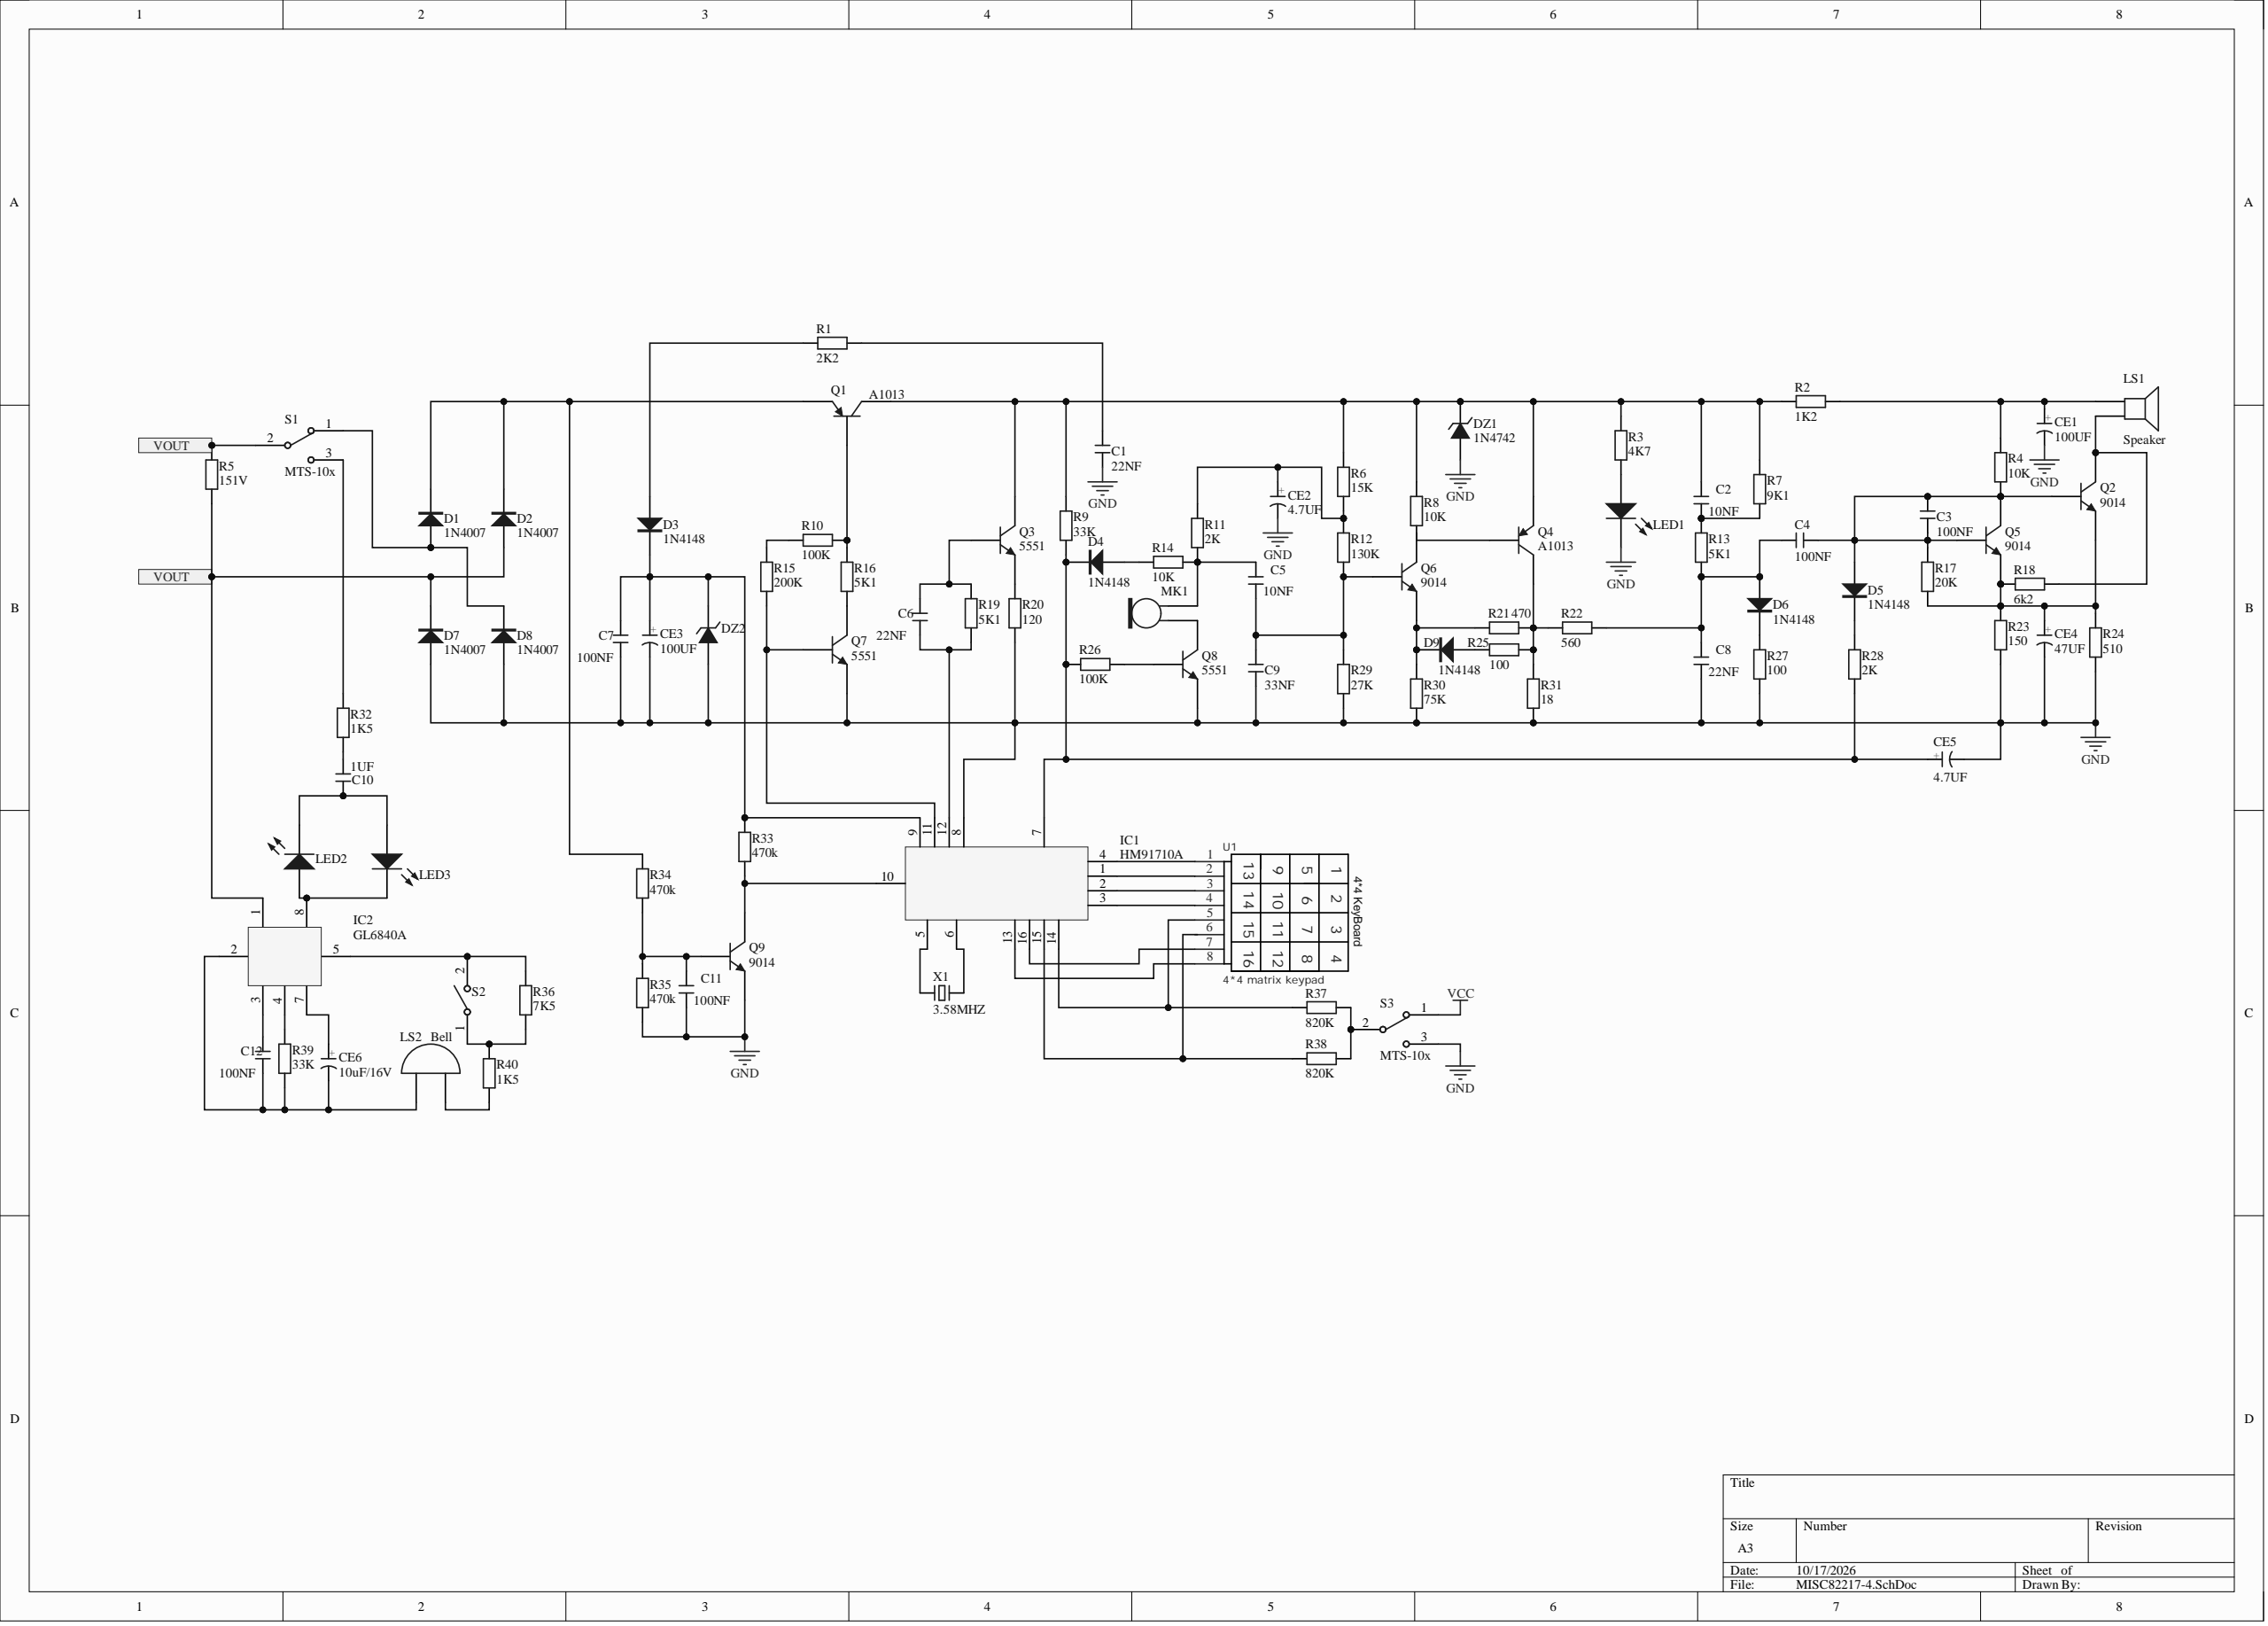Circuit board | Altium Designer | 91 parts | 59 nets
Bill of materials:
Comment,Description,Designator,Footprint,LibRef,Quantity
"22NF","Ceramic disc capacitor","C1, C6, C8","CC 2.2*5","CC","3"
"10NF","Ceramic disc capacitor","C2, C5","CC 2.2*5","CC","2"
"100NF","Ceramic disc capacitor","C3, C4, C7, C11, C12","CC 2.2*5","CC","5"
"33NF","Ceramic disc capacitor","C9","CC 2.2*5","CC","1"
"1UF","Ceramic disc capacitor","C10","CC 2.2*5","CC","1"
"100UF","Through-hole electrolytic capacitor","CE1, CE3","CAP 1.5*4*8","CE","2"
"4.7UF","Through-hole electrolytic capacitor","CE2, CE5","CAP 1.5*4*8","CE","2"
"47UF","Through-hole electrolytic capacitor","CE4","CAP 1.5*4*8","CE","1"
"10uF/16V","Through-hole electrolytic capacitor","CE6","CAP 1.5*4*8","CE","1"
"1N4007","Rectifier diode","D1, D2, D7, D8","DO-41","1N4007","4"
"1N4148","Switching diode","D3, D4, D5, D6, D9","MINI_MELF (LL34)","1N4148","5"
"1N4742","5.1V/1W Zener diode","DZ1","DO-41","1N4733","1"
"1N4106","12V/0.5W Zener diode","DZ2","DO-35","1N4106","1"
"HM91710A","","IC1","DIP16","HM91710A","1"
"GL6840A","","IC2","DIP8","GL6840A","1"
"Red","Through-hole 3mm LED","LED1, LED2, LED3","LED 3MM-B","LED-3MM","3"
"Speaker","Loudspeaker","LS1","PIN2","Speaker","1"
"Bell","Electrical Bell","LS2","PIN2","Bell","1"
"Mic2","Microphone","MK1","PIN2","Mic2","1"
"A1013","PNP General Purpose Amplifier","Q1, Q4","TO-92A","2N3906","2"
"9014","NPN General Purpose Amplifier","Q2, Q5, Q6, Q9","TO-92A","2N3904","4"
"5551","NPN General Purpose Amplifier","Q3, Q7, Q8","TO-92A","2N3904","3"
"2K2","Color-band resistor","R1","RS 1/4W","R-S","1"
"1K2","Color-band resistor","R2","RS 1/4W","R-S","1"
"4K7","Color-band resistor","R3","RS 1/4W","R-S","1"
"10K","Color-band resistor","R4, R8, R14","RS 1/4W","R-S","3"
"151V","Color-band resistor","R5","RS 1/4W","R-S","1"
"15K","Color-band resistor","R6","RS 1/4W","R-S","1"
"9K1","Color-band resistor","R7","RS 1/4W","R-S","1"
"33K","Color-band resistor","R9, R39","RS 1/4W","R-S","2"
"100K","Color-band resistor","R10, R26","RS 1/4W","R-S","2"
"2K","Color-band resistor","R11, R28","RS 1/4W","R-S","2"
"130K","Color-band resistor","R12","RS 1/4W","R-S","1"
"5K1","Color-band resistor","R13, R16, R19","RS 1/4W","R-S","3"
"200K","Color-band resistor","R15","RS 1/4W","R-S","1"
"20K","Color-band resistor","R17","RS 1/4W","R-S","1"
"6k2","Color-band resistor","R18","RS 1/4W","R-S","1"
"120","Color-band resistor","R20","RS 1/4W","R-S","1"
"470","Color-band resistor","R21","RS 1/4W","R-S","1"
"560","Color-band resistor","R22","RS 1/4W","R-S","1"
"150","Color-band resistor","R23","RS 1/4W","R-S","1"
"510","Color-band resistor","R24","RS 1/4W","R-S","1"
"100","Color-band resistor","R25, R27","RS 1/4W","R-S","2"
"27K","Color-band resistor","R29","RS 1/4W","R-S","1"
"75K","Color-band resistor","R30","RS 1/4W","R-S","1"
"18","Color-band resistor","R31","RS 1/4W","R-S","1"
"1K5","Color-band resistor","R32, R40","RS 1/4W","R-S","2"
"470k","Color-band resistor","R33, R34, R35","RS 1/4W","R-S","3"
"7K5","Color-band resistor","R36","RS 1/4W","R-S","1"
"820K","Color-band resistor","R37, R38","RS 1/4W","R-S","2"
"MTS-10x","MTS10x series 3-pin twist switch","S1, S3","MTS-10x","MTS-10x","2"
"KCD1-101","1-way SPST boat-type switch","S2","KCD1-101","KCD1-101","1"
"4*4 matrix keypad","","U1","4*4 KEYBOARD","4*4矩阵键盘","1"
"3.58MHZ","2-pin passive crystal","X1","OSC HC-49S","XTAL-2P","1"
Netlist (Protel format):
[
C1
CC 2.2*5
22NF



]
[
C2
CC 2.2*5
10NF



]
[
C3
CC 2.2*5
100NF



]
[
C4
CC 2.2*5
100NF



]
[
C5
CC 2.2*5
10NF



]
[
C6
CC 2.2*5
22NF



]
[
C7
CC 2.2*5
100NF



]
[
C8
CC 2.2*5
22NF



]
[
C9
CC 2.2*5
33NF



]
[
C10
CC 2.2*5
1UF



]
[
C11
CC 2.2*5
100NF



]
[
C12
CC 2.2*5
100NF



]
[
CE1
CAP 1.5*4*8
100UF



]
[
CE2
CAP 1.5*4*8
4.7UF



]
[
CE3
CAP 1.5*4*8
100UF



]
[
CE4
CAP 1.5*4*8
47UF



]
[
CE5
CAP 1.5*4*8
4.7UF



]
[
CE6
CAP 1.5*4*8
10uF/16V



]
[
D1
DO-41
1N4007



]
[
D2
DO-41
1N4007



]
[
D3
MINI_MELF (LL34)
1N4148



]
[
D4
MINI_MELF (LL34)
1N4148



]
[
D5
MINI_MELF (LL34)
1N4148



]
[
D6
MINI_MELF (LL34)
1N4148



]
[
D7
DO-41
1N4007



]
[
D8
DO-41
1N4007



]
[
D9
MINI_MELF (LL34)
1N4148



]
[
DZ1
DO-41
1N4742



]
[
DZ2
DO-35
1N4106



]
[
IC1
DIP16
HM91710A



]
[
IC2
DIP8
GL6840A



]
[
LED1
LED 3MM-B
Red



]
[
LED2
LED 3MM-B
Red



]
[
LED3
LED 3MM-B
Red



]
[
LS1
PIN2
Speaker



]
[
LS2
PIN2
Bell



]
[
MK1
PIN2
Mic2



]
[
Q1
TO-92A
A1013



]
[
Q2
TO-92A
9014



]
[
Q3
TO-92A
5551



]
[
Q4
TO-92A
A1013



]
[
Q5
TO-92A
9014



]
[
Q6
TO-92A
9014



]
[
Q7
TO-92A
5551



]
[
Q8
TO-92A
5551



]
[
Q9
TO-92A
9014



]
[
R1
RS 1/4W
2K2



]
[
R2
RS 1/4W
1K2



]
[
R3
RS 1/4W
4K7



]
[
R4
RS 1/4W
10K



]
[
R5
RS 1/4W
151V



]
[
R6
RS 1/4W
15K



]
[
R7
RS 1/4W
9K1



]
[
R8
RS 1/4W
10K



]
[
R9
RS 1/4W
33K



]
[
R10
RS 1/4W
100K



]
[
R11
RS 1/4W
2K



]
[
R12
RS 1/4W
130K



]
[
R13
RS 1/4W
5K1



]
[
R14
RS 1/4W
10K



]
[
R15
RS 1/4W
200K



]
[
R16
RS 1/4W
5K1



]
[
R17
RS 1/4W
20K



]
[
R18
RS 1/4W
6k2



]
[
R19
RS 1/4W
5K1



]
[
R20
RS 1/4W
120



]
[
R21
RS 1/4W
470



]
[
R22
RS 1/4W
560



]
[
R23
RS 1/4W
150



]
[
R24
RS 1/4W
510



]
[
R25
RS 1/4W
100



]
[
R26
RS 1/4W
100K



]
[
R27
RS 1/4W
100



]
[
R28
RS 1/4W
2K



]
[
R29
RS 1/4W
27K



]
[
R30
RS 1/4W
75K



]
[
R31
RS 1/4W
18



]
[
R32
RS 1/4W
1K5



]
[
R33
RS 1/4W
470k



]
[
R34
RS 1/4W
470k



]
[
R35
RS 1/4W
470k



]
[
R36
RS 1/4W
7K5



]
[
R37
RS 1/4W
820K



]
[
R38
RS 1/4W
820K



]
[
R39
RS 1/4W
33K



]
[
R40
RS 1/4W
1K5



]
[
S1
MTS-10x
MTS-10x



]
[
S2
KCD1-101
KCD1-101



]
[
S3
MTS-10x
MTS-10x



]
[
U1
4*4 KEYBOARD
4*4 matrix keypad



]
[
X1
OSC HC-49S
3.58MHZ



]
(
NetR37_1
R37-1
R38-1
S3-2
)
(
NetR36_1
R36-1
R40-2
S2-1
)
(
NetR32_2
R32-2
S1-3
)
(
NetR10_2
R10-2
R15-1
)
(
NetQ8_2
Q8-2
R26-1
)
(
NetQ7_3
Q7-3
R16-1
)
(
NetQ4_3
Q4-3
R21-2
R22-2
R25-2
R31-2
)
(
NetQ4_2
Q4-2
R8-2
)
(
NetQ3_1
Q3-1
R20-2
)
(
NetQ1_2
Q1-2
R10-1
R16-2
)
(
NetMK1_2
MK1-2
Q8-3
)
(
NetLS2_2
LS2-2
R40-1
)
(
NetLS1_2
LS1-2
Q2-3
R18-1
)
(
NetLED1_1
LED1-1
R3-2
)
(
NetIC2_8
IC2-8
LED2-1
LED3-2
)
(
NetIC2_5
IC2-5
R36-2
S2-2
)
(
NetIC2_4
IC2-4
R39-2
)
(
NetIC1_16
IC1-16
U1-7
)
(
NetIC1_15
IC1-15
R38-2
)
(
NetIC1_14
IC1-14
R37-2
U1-5
)
(
NetIC1_13
IC1-13
U1-8
)
(
NetIC1_11
IC1-11
Q7-2
R15-2
)
(
NetIC1_10
IC1-10
Q9-3
R33-1
)
(
NetIC1_6
IC1-6
X1-2
)
(
NetIC1_5
IC1-5
X1-1
)
(
NetIC1_4
IC1-4
U1-1
)
(
NetIC1_3
IC1-3
U1-4
)
(
NetIC1_2
IC1-2
U1-3
)
(
NetIC1_1
IC1-1
U1-2
)
(
NetD9_2
D9-2
Q6-1
R21-1
R30-1
)
(
NetD9_1
D9-1
R25-1
)
(
NetD6_2
D6-2
R27-1
)
(
NetD5_2
D5-2
R28-1
)
(
NetD4_1
D4-1
R14-2
)
(
NetD3_1
D3-1
R1-2
)
(
NetD2_1
D2-1
D7-2
IC2-1
R5-1
R5-2
S1-2
)
(
NetD1_2
D1-2
D2-2
Q1-1
R34-2
)
(
NetD1_1
D1-1
D8-2
S1-1
)
(
NetCE6_1
CE6-1
IC2-7
)
(
NetCE5_1
CE5-1
D4-2
IC1-7
R9-1
R26-2
R28-2
)
(
NetCE4_1
CE4-1
Q2-1
Q5-1
R17-1
R18-2
R23-2
R24-2
)
(
NetCE2_1
CE2-1
R6-2
R11-1
R12-1
)
(
NetCE1_1
CE1-1
LS1-1
R2-2
R4-2
)
(
NetC12_2
C12-2
IC2-3
)
(
NetC12_1
C12-1
CE6-2
IC2-2
LS2-1
R39-1
)
(
NetC11_2
C11-2
Q9-2
R34-1
R35-2
)
(
NetC10_2
C10-2
LED2-2
LED3-1
)
(
NetC10_1
C10-1
R32-1
)
(
NetC7_2
C7-2
CE3-1
D3-2
DZ2-2
IC1-9
R33-2
)
(
NetC6_2
C6-2
Q3-2
R19-2
)
(
NetC6_1
C6-1
IC1-12
R19-1
)
(
NetC5_2
C5-2
MK1-1
R11-2
R14-1
)
(
NetC5_1
C5-1
C9-2
Q6-2
R12-2
R29-1
)
(
NetC4_2
C4-2
C8-2
D6-1
R13-2
R22-1
)
(
NetC3_1
C3-1
C3-2
C4-1
D5-1
Q2-2
Q5-2
Q5-3
R4-1
R17-2
)
(
NetC2_2
C2-2
DZ1-2
Q1-3
Q3-3
Q4-1
R2-1
R3-1
R6-1
R7-1
R8-1
R9-2
)
(
NetC2_1
C2-1
R7-2
R13-1
)
(
NetC1_2
C1-2
R1-1
)
(
GND
C1-1
C7-1
C8-1
C9-1
C11-1
CE1-2
CE2-2
CE3-2
CE4-2
CE5-2
D7-1
D8-1
DZ1-1
DZ2-1
IC1-8
LED1-2
Q7-1
Q8-1
Q9-1
R20-1
R23-1
R24-1
R27-2
R29-2
R30-2
R31-1
R35-1
S3-3
)